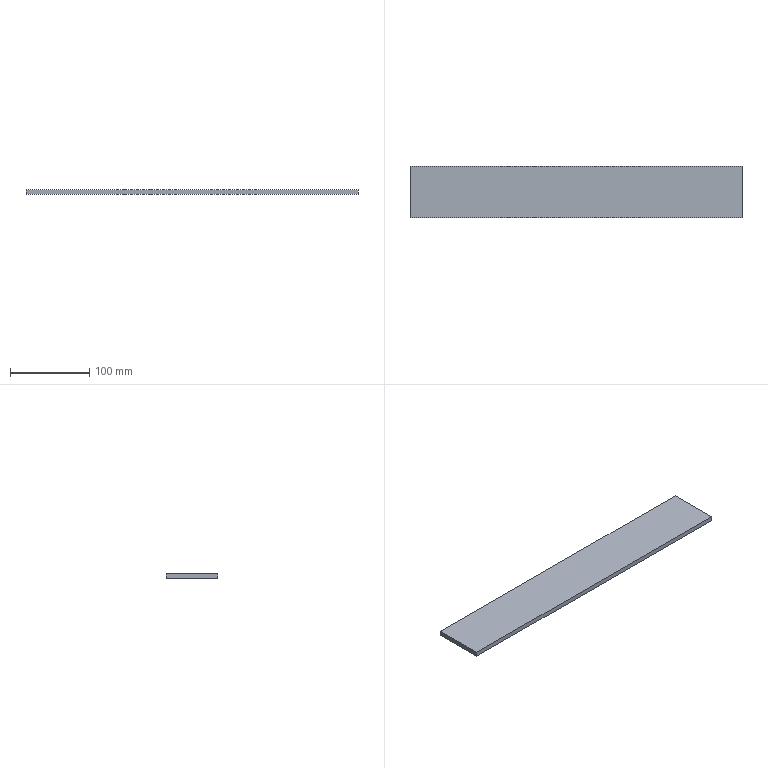Part | STEP file | 03-Support plate | 1 solid | 6 faces | box 420 x 65 x 6 mm | volume 163800 mm3 | plane 6
STEP:
#1=CARTESIAN_POINT('',(0.,0.,0.));
#2=DIRECTION('',(0.,0.,1.));
#3=DIRECTION('',(1.,0.,0.));
#4=AXIS2_PLACEMENT_3D('',#1,#2,#3);
#5=CARTESIAN_POINT('',(0.,0.,0.));
#6=VERTEX_POINT('',#5);
#7=CARTESIAN_POINT('',(0.,-65.,0.));
#8=VERTEX_POINT('',#7);
#9=CARTESIAN_POINT('',(0.,0.,0.));
#10=DIRECTION('',(0.,-1.,0.));
#11=VECTOR('',#10,1.);
#12=LINE('',#9,#11);
#13=CARTESIAN_POINT('',(0.,0.,6.));
#14=DIRECTION('',(1.,0.,0.));
#15=DIRECTION('',(0.,1.,0.));
#16=AXIS2_PLACEMENT_3D('',#13,#14,#15);
#17=PLANE('',#16);
#18=CARTESIAN_POINT('',(0.,-6.));
#19=DIRECTION('',(-1.,0.));
#20=VECTOR('',#19,1.);
#21=LINE('',#18,#20);
#22=(GEOMETRIC_REPRESENTATION_CONTEXT(2)PARAMETRIC_REPRESENTATION_CONTEXT()REPRESENTATION_CONTEXT('',''));
#23=DEFINITIONAL_REPRESENTATION('',(#21),#22);
#24=PCURVE('',#17,#23);
#25=CARTESIAN_POINT('',(0.,0.,0.));
#26=DIRECTION('',(0.,0.,1.));
#27=DIRECTION('',(1.,0.,0.));
#28=AXIS2_PLACEMENT_3D('',#25,#26,#27);
#29=PLANE('',#28);
#30=CARTESIAN_POINT('',(0.,0.));
#31=DIRECTION('',(0.,-1.));
#32=VECTOR('',#31,1.);
#33=LINE('',#30,#32);
#34=(GEOMETRIC_REPRESENTATION_CONTEXT(2)PARAMETRIC_REPRESENTATION_CONTEXT()REPRESENTATION_CONTEXT('',''));
#35=DEFINITIONAL_REPRESENTATION('',(#33),#34);
#36=PCURVE('',#29,#35);
#37=SURFACE_CURVE('',#12,(#24,#36),.PCURVE_S1.);
#38=EDGE_CURVE('',#6,#8,#37,.T.);
#39=ORIENTED_EDGE('',*,*,#38,.T.);
#40=CARTESIAN_POINT('',(0.,-65.,6.));
#41=VERTEX_POINT('',#40);
#42=CARTESIAN_POINT('',(0.,-65.,6.));
#43=DIRECTION('',(0.,0.,-1.));
#44=VECTOR('',#43,1.);
#45=LINE('',#42,#44);
#46=CARTESIAN_POINT('',(-65.,0.));
#47=DIRECTION('',(0.,-1.));
#48=VECTOR('',#47,1.);
#49=LINE('',#46,#48);
#50=(GEOMETRIC_REPRESENTATION_CONTEXT(2)PARAMETRIC_REPRESENTATION_CONTEXT()REPRESENTATION_CONTEXT('',''));
#51=DEFINITIONAL_REPRESENTATION('',(#49),#50);
#52=PCURVE('',#17,#51);
#53=CARTESIAN_POINT('',(0.,-65.,6.));
#54=DIRECTION('',(0.,1.,0.));
#55=DIRECTION('',(0.,0.,1.));
#56=AXIS2_PLACEMENT_3D('',#53,#54,#55);
#57=PLANE('',#56);
#58=CARTESIAN_POINT('',(0.,0.));
#59=DIRECTION('',(-1.,0.));
#60=VECTOR('',#59,1.);
#61=LINE('',#58,#60);
#62=(GEOMETRIC_REPRESENTATION_CONTEXT(2)PARAMETRIC_REPRESENTATION_CONTEXT()REPRESENTATION_CONTEXT('',''));
#63=DEFINITIONAL_REPRESENTATION('',(#61),#62);
#64=PCURVE('',#57,#63);
#65=SURFACE_CURVE('',#45,(#52,#64),.PCURVE_S1.);
#66=EDGE_CURVE('',#41,#8,#65,.T.);
#67=ORIENTED_EDGE('',*,*,#66,.F.);
#68=CARTESIAN_POINT('',(0.,0.,6.));
#69=VERTEX_POINT('',#68);
#70=CARTESIAN_POINT('',(0.,0.,6.));
#71=DIRECTION('',(0.,-1.,0.));
#72=VECTOR('',#71,1.);
#73=LINE('',#70,#72);
#74=CARTESIAN_POINT('',(0.,0.));
#75=DIRECTION('',(-1.,0.));
#76=VECTOR('',#75,1.);
#77=LINE('',#74,#76);
#78=(GEOMETRIC_REPRESENTATION_CONTEXT(2)PARAMETRIC_REPRESENTATION_CONTEXT()REPRESENTATION_CONTEXT('',''));
#79=DEFINITIONAL_REPRESENTATION('',(#77),#78);
#80=PCURVE('',#17,#79);
#81=CARTESIAN_POINT('',(0.,0.,6.));
#82=DIRECTION('',(0.,0.,1.));
#83=DIRECTION('',(1.,0.,0.));
#84=AXIS2_PLACEMENT_3D('',#81,#82,#83);
#85=PLANE('',#84);
#86=CARTESIAN_POINT('',(0.,0.));
#87=DIRECTION('',(0.,-1.));
#88=VECTOR('',#87,1.);
#89=LINE('',#86,#88);
#90=(GEOMETRIC_REPRESENTATION_CONTEXT(2)PARAMETRIC_REPRESENTATION_CONTEXT()REPRESENTATION_CONTEXT('',''));
#91=DEFINITIONAL_REPRESENTATION('',(#89),#90);
#92=PCURVE('',#85,#91);
#93=SURFACE_CURVE('',#73,(#80,#92),.PCURVE_S1.);
#94=EDGE_CURVE('',#69,#41,#93,.T.);
#95=ORIENTED_EDGE('',*,*,#94,.F.);
#96=CARTESIAN_POINT('',(0.,0.,6.));
#97=DIRECTION('',(0.,0.,-1.));
#98=VECTOR('',#97,1.);
#99=LINE('',#96,#98);
#100=CARTESIAN_POINT('',(0.,0.));
#101=DIRECTION('',(0.,-1.));
#102=VECTOR('',#101,1.);
#103=LINE('',#100,#102);
#104=(GEOMETRIC_REPRESENTATION_CONTEXT(2)PARAMETRIC_REPRESENTATION_CONTEXT()REPRESENTATION_CONTEXT('',''));
#105=DEFINITIONAL_REPRESENTATION('',(#103),#104);
#106=PCURVE('',#17,#105);
#107=CARTESIAN_POINT('',(0.,0.,6.));
#108=DIRECTION('',(0.,-1.,0.));
#109=DIRECTION('',(0.,0.,-1.));
#110=AXIS2_PLACEMENT_3D('',#107,#108,#109);
#111=PLANE('',#110);
#112=CARTESIAN_POINT('',(0.,0.));
#113=DIRECTION('',(1.,0.));
#114=VECTOR('',#113,1.);
#115=LINE('',#112,#114);
#116=(GEOMETRIC_REPRESENTATION_CONTEXT(2)PARAMETRIC_REPRESENTATION_CONTEXT()REPRESENTATION_CONTEXT('',''));
#117=DEFINITIONAL_REPRESENTATION('',(#115),#116);
#118=PCURVE('',#111,#117);
#119=SURFACE_CURVE('',#99,(#106,#118),.PCURVE_S1.);
#120=EDGE_CURVE('',#69,#6,#119,.T.);
#121=ORIENTED_EDGE('',*,*,#120,.T.);
#122=EDGE_LOOP('',(#39,#67,#95,#121));
#123=FACE_BOUND('',#122,.T.);
#124=ADVANCED_FACE('',(#123),#17,.F.);
#125=CARTESIAN_POINT('',(420.,-65.,0.));
#126=VERTEX_POINT('',#125);
#127=CARTESIAN_POINT('',(0.,-65.,0.));
#128=DIRECTION('',(1.,0.,0.));
#129=VECTOR('',#128,1.);
#130=LINE('',#127,#129);
#131=CARTESIAN_POINT('',(-6.,0.));
#132=DIRECTION('',(0.,1.));
#133=VECTOR('',#132,1.);
#134=LINE('',#131,#133);
#135=(GEOMETRIC_REPRESENTATION_CONTEXT(2)PARAMETRIC_REPRESENTATION_CONTEXT()REPRESENTATION_CONTEXT('',''));
#136=DEFINITIONAL_REPRESENTATION('',(#134),#135);
#137=PCURVE('',#57,#136);
#138=CARTESIAN_POINT('',(0.,-65.));
#139=DIRECTION('',(1.,0.));
#140=VECTOR('',#139,1.);
#141=LINE('',#138,#140);
#142=(GEOMETRIC_REPRESENTATION_CONTEXT(2)PARAMETRIC_REPRESENTATION_CONTEXT()REPRESENTATION_CONTEXT('',''));
#143=DEFINITIONAL_REPRESENTATION('',(#141),#142);
#144=PCURVE('',#29,#143);
#145=SURFACE_CURVE('',#130,(#137,#144),.PCURVE_S1.);
#146=EDGE_CURVE('',#8,#126,#145,.T.);
#147=ORIENTED_EDGE('',*,*,#146,.T.);
#148=CARTESIAN_POINT('',(420.,-65.,6.));
#149=VERTEX_POINT('',#148);
#150=CARTESIAN_POINT('',(420.,-65.,6.));
#151=DIRECTION('',(0.,0.,-1.));
#152=VECTOR('',#151,1.);
#153=LINE('',#150,#152);
#154=CARTESIAN_POINT('',(0.,420.));
#155=DIRECTION('',(-1.,0.));
#156=VECTOR('',#155,1.);
#157=LINE('',#154,#156);
#158=(GEOMETRIC_REPRESENTATION_CONTEXT(2)PARAMETRIC_REPRESENTATION_CONTEXT()REPRESENTATION_CONTEXT('',''));
#159=DEFINITIONAL_REPRESENTATION('',(#157),#158);
#160=PCURVE('',#57,#159);
#161=CARTESIAN_POINT('',(420.,0.,6.));
#162=DIRECTION('',(-1.,0.,0.));
#163=DIRECTION('',(0.,-1.,0.));
#164=AXIS2_PLACEMENT_3D('',#161,#162,#163);
#165=PLANE('',#164);
#166=CARTESIAN_POINT('',(65.,0.));
#167=DIRECTION('',(0.,-1.));
#168=VECTOR('',#167,1.);
#169=LINE('',#166,#168);
#170=(GEOMETRIC_REPRESENTATION_CONTEXT(2)PARAMETRIC_REPRESENTATION_CONTEXT()REPRESENTATION_CONTEXT('',''));
#171=DEFINITIONAL_REPRESENTATION('',(#169),#170);
#172=PCURVE('',#165,#171);
#173=SURFACE_CURVE('',#153,(#160,#172),.PCURVE_S1.);
#174=EDGE_CURVE('',#149,#126,#173,.T.);
#175=ORIENTED_EDGE('',*,*,#174,.F.);
#176=CARTESIAN_POINT('',(0.,-65.,6.));
#177=DIRECTION('',(1.,0.,0.));
#178=VECTOR('',#177,1.);
#179=LINE('',#176,#178);
#180=CARTESIAN_POINT('',(0.,0.));
#181=DIRECTION('',(0.,1.));
#182=VECTOR('',#181,1.);
#183=LINE('',#180,#182);
#184=(GEOMETRIC_REPRESENTATION_CONTEXT(2)PARAMETRIC_REPRESENTATION_CONTEXT()REPRESENTATION_CONTEXT('',''));
#185=DEFINITIONAL_REPRESENTATION('',(#183),#184);
#186=PCURVE('',#57,#185);
#187=CARTESIAN_POINT('',(0.,-65.));
#188=DIRECTION('',(1.,0.));
#189=VECTOR('',#188,1.);
#190=LINE('',#187,#189);
#191=(GEOMETRIC_REPRESENTATION_CONTEXT(2)PARAMETRIC_REPRESENTATION_CONTEXT()REPRESENTATION_CONTEXT('',''));
#192=DEFINITIONAL_REPRESENTATION('',(#190),#191);
#193=PCURVE('',#85,#192);
#194=SURFACE_CURVE('',#179,(#186,#193),.PCURVE_S1.);
#195=EDGE_CURVE('',#41,#149,#194,.T.);
#196=ORIENTED_EDGE('',*,*,#195,.F.);
#197=ORIENTED_EDGE('',*,*,#66,.T.);
#198=EDGE_LOOP('',(#147,#175,#196,#197));
#199=FACE_BOUND('',#198,.T.);
#200=ADVANCED_FACE('',(#199),#57,.F.);
#201=CARTESIAN_POINT('',(420.,0.,0.));
#202=VERTEX_POINT('',#201);
#203=CARTESIAN_POINT('',(420.,0.,0.));
#204=DIRECTION('',(0.,1.,0.));
#205=VECTOR('',#204,1.);
#206=LINE('',#203,#205);
#207=CARTESIAN_POINT('',(0.,-6.));
#208=DIRECTION('',(-1.,0.));
#209=VECTOR('',#208,1.);
#210=LINE('',#207,#209);
#211=(GEOMETRIC_REPRESENTATION_CONTEXT(2)PARAMETRIC_REPRESENTATION_CONTEXT()REPRESENTATION_CONTEXT('',''));
#212=DEFINITIONAL_REPRESENTATION('',(#210),#211);
#213=PCURVE('',#165,#212);
#214=CARTESIAN_POINT('',(420.,0.));
#215=DIRECTION('',(0.,1.));
#216=VECTOR('',#215,1.);
#217=LINE('',#214,#216);
#218=(GEOMETRIC_REPRESENTATION_CONTEXT(2)PARAMETRIC_REPRESENTATION_CONTEXT()REPRESENTATION_CONTEXT('',''));
#219=DEFINITIONAL_REPRESENTATION('',(#217),#218);
#220=PCURVE('',#29,#219);
#221=SURFACE_CURVE('',#206,(#213,#220),.PCURVE_S1.);
#222=EDGE_CURVE('',#126,#202,#221,.T.);
#223=ORIENTED_EDGE('',*,*,#222,.T.);
#224=CARTESIAN_POINT('',(420.,0.,6.));
#225=VERTEX_POINT('',#224);
#226=CARTESIAN_POINT('',(420.,0.,6.));
#227=DIRECTION('',(0.,0.,-1.));
#228=VECTOR('',#227,1.);
#229=LINE('',#226,#228);
#230=CARTESIAN_POINT('',(0.,0.));
#231=DIRECTION('',(0.,-1.));
#232=VECTOR('',#231,1.);
#233=LINE('',#230,#232);
#234=(GEOMETRIC_REPRESENTATION_CONTEXT(2)PARAMETRIC_REPRESENTATION_CONTEXT()REPRESENTATION_CONTEXT('',''));
#235=DEFINITIONAL_REPRESENTATION('',(#233),#234);
#236=PCURVE('',#165,#235);
#237=CARTESIAN_POINT('',(0.,420.));
#238=DIRECTION('',(1.,0.));
#239=VECTOR('',#238,1.);
#240=LINE('',#237,#239);
#241=(GEOMETRIC_REPRESENTATION_CONTEXT(2)PARAMETRIC_REPRESENTATION_CONTEXT()REPRESENTATION_CONTEXT('',''));
#242=DEFINITIONAL_REPRESENTATION('',(#240),#241);
#243=PCURVE('',#111,#242);
#244=SURFACE_CURVE('',#229,(#236,#243),.PCURVE_S1.);
#245=EDGE_CURVE('',#225,#202,#244,.T.);
#246=ORIENTED_EDGE('',*,*,#245,.F.);
#247=CARTESIAN_POINT('',(420.,0.,6.));
#248=DIRECTION('',(0.,1.,0.));
#249=VECTOR('',#248,1.);
#250=LINE('',#247,#249);
#251=CARTESIAN_POINT('',(0.,0.));
#252=DIRECTION('',(-1.,0.));
#253=VECTOR('',#252,1.);
#254=LINE('',#251,#253);
#255=(GEOMETRIC_REPRESENTATION_CONTEXT(2)PARAMETRIC_REPRESENTATION_CONTEXT()REPRESENTATION_CONTEXT('',''));
#256=DEFINITIONAL_REPRESENTATION('',(#254),#255);
#257=PCURVE('',#165,#256);
#258=CARTESIAN_POINT('',(420.,0.));
#259=DIRECTION('',(0.,1.));
#260=VECTOR('',#259,1.);
#261=LINE('',#258,#260);
#262=(GEOMETRIC_REPRESENTATION_CONTEXT(2)PARAMETRIC_REPRESENTATION_CONTEXT()REPRESENTATION_CONTEXT('',''));
#263=DEFINITIONAL_REPRESENTATION('',(#261),#262);
#264=PCURVE('',#85,#263);
#265=SURFACE_CURVE('',#250,(#257,#264),.PCURVE_S1.);
#266=EDGE_CURVE('',#149,#225,#265,.T.);
#267=ORIENTED_EDGE('',*,*,#266,.F.);
#268=ORIENTED_EDGE('',*,*,#174,.T.);
#269=EDGE_LOOP('',(#223,#246,#267,#268));
#270=FACE_BOUND('',#269,.T.);
#271=ADVANCED_FACE('',(#270),#165,.F.);
#272=CARTESIAN_POINT('',(0.,0.,0.));
#273=DIRECTION('',(-1.,0.,0.));
#274=VECTOR('',#273,1.);
#275=LINE('',#272,#274);
#276=CARTESIAN_POINT('',(6.,0.));
#277=DIRECTION('',(0.,-1.));
#278=VECTOR('',#277,1.);
#279=LINE('',#276,#278);
#280=(GEOMETRIC_REPRESENTATION_CONTEXT(2)PARAMETRIC_REPRESENTATION_CONTEXT()REPRESENTATION_CONTEXT('',''));
#281=DEFINITIONAL_REPRESENTATION('',(#279),#280);
#282=PCURVE('',#111,#281);
#283=CARTESIAN_POINT('',(0.,0.));
#284=DIRECTION('',(-1.,0.));
#285=VECTOR('',#284,1.);
#286=LINE('',#283,#285);
#287=(GEOMETRIC_REPRESENTATION_CONTEXT(2)PARAMETRIC_REPRESENTATION_CONTEXT()REPRESENTATION_CONTEXT('',''));
#288=DEFINITIONAL_REPRESENTATION('',(#286),#287);
#289=PCURVE('',#29,#288);
#290=SURFACE_CURVE('',#275,(#282,#289),.PCURVE_S1.);
#291=EDGE_CURVE('',#202,#6,#290,.T.);
#292=ORIENTED_EDGE('',*,*,#291,.T.);
#293=ORIENTED_EDGE('',*,*,#120,.F.);
#294=CARTESIAN_POINT('',(0.,0.,6.));
#295=DIRECTION('',(-1.,0.,0.));
#296=VECTOR('',#295,1.);
#297=LINE('',#294,#296);
#298=CARTESIAN_POINT('',(0.,0.));
#299=DIRECTION('',(0.,-1.));
#300=VECTOR('',#299,1.);
#301=LINE('',#298,#300);
#302=(GEOMETRIC_REPRESENTATION_CONTEXT(2)PARAMETRIC_REPRESENTATION_CONTEXT()REPRESENTATION_CONTEXT('',''));
#303=DEFINITIONAL_REPRESENTATION('',(#301),#302);
#304=PCURVE('',#111,#303);
#305=CARTESIAN_POINT('',(0.,0.));
#306=DIRECTION('',(-1.,0.));
#307=VECTOR('',#306,1.);
#308=LINE('',#305,#307);
#309=(GEOMETRIC_REPRESENTATION_CONTEXT(2)PARAMETRIC_REPRESENTATION_CONTEXT()REPRESENTATION_CONTEXT('',''));
#310=DEFINITIONAL_REPRESENTATION('',(#308),#309);
#311=PCURVE('',#85,#310);
#312=SURFACE_CURVE('',#297,(#304,#311),.PCURVE_S1.);
#313=EDGE_CURVE('',#225,#69,#312,.T.);
#314=ORIENTED_EDGE('',*,*,#313,.F.);
#315=ORIENTED_EDGE('',*,*,#245,.T.);
#316=EDGE_LOOP('',(#292,#293,#314,#315));
#317=FACE_BOUND('',#316,.T.);
#318=ADVANCED_FACE('',(#317),#111,.F.);
#319=ORIENTED_EDGE('',*,*,#94,.T.);
#320=ORIENTED_EDGE('',*,*,#195,.T.);
#321=ORIENTED_EDGE('',*,*,#266,.T.);
#322=ORIENTED_EDGE('',*,*,#313,.T.);
#323=EDGE_LOOP('',(#319,#320,#321,#322));
#324=FACE_BOUND('',#323,.T.);
#325=ADVANCED_FACE('',(#324),#85,.T.);
#326=ORIENTED_EDGE('',*,*,#38,.F.);
#327=ORIENTED_EDGE('',*,*,#291,.F.);
#328=ORIENTED_EDGE('',*,*,#222,.F.);
#329=ORIENTED_EDGE('',*,*,#146,.F.);
#330=EDGE_LOOP('',(#326,#327,#328,#329));
#331=FACE_BOUND('',#330,.T.);
#332=ADVANCED_FACE('',(#331),#29,.F.);
#333=CLOSED_SHELL('',(#124,#200,#271,#318,#325,#332));
#334=MANIFOLD_SOLID_BREP('',#333);
#335=(LENGTH_UNIT()NAMED_UNIT(*)SI_UNIT(.MILLI.,.METRE.));
#336=UNCERTAINTY_MEASURE_WITH_UNIT(LENGTH_MEASURE(0.0000001),#335,'','');
#337=(NAMED_UNIT(*)PLANE_ANGLE_UNIT()SI_UNIT($,.RADIAN.));
#338=(NAMED_UNIT(*)SI_UNIT($,.STERADIAN.)SOLID_ANGLE_UNIT());
#339=(GEOMETRIC_REPRESENTATION_CONTEXT(3)GLOBAL_UNCERTAINTY_ASSIGNED_CONTEXT((#336))GLOBAL_UNIT_ASSIGNED_CONTEXT((#335,#337,#338))REPRESENTATION_CONTEXT('',''));
#340=ADVANCED_BREP_SHAPE_REPRESENTATION('',(#4,#334),#339);